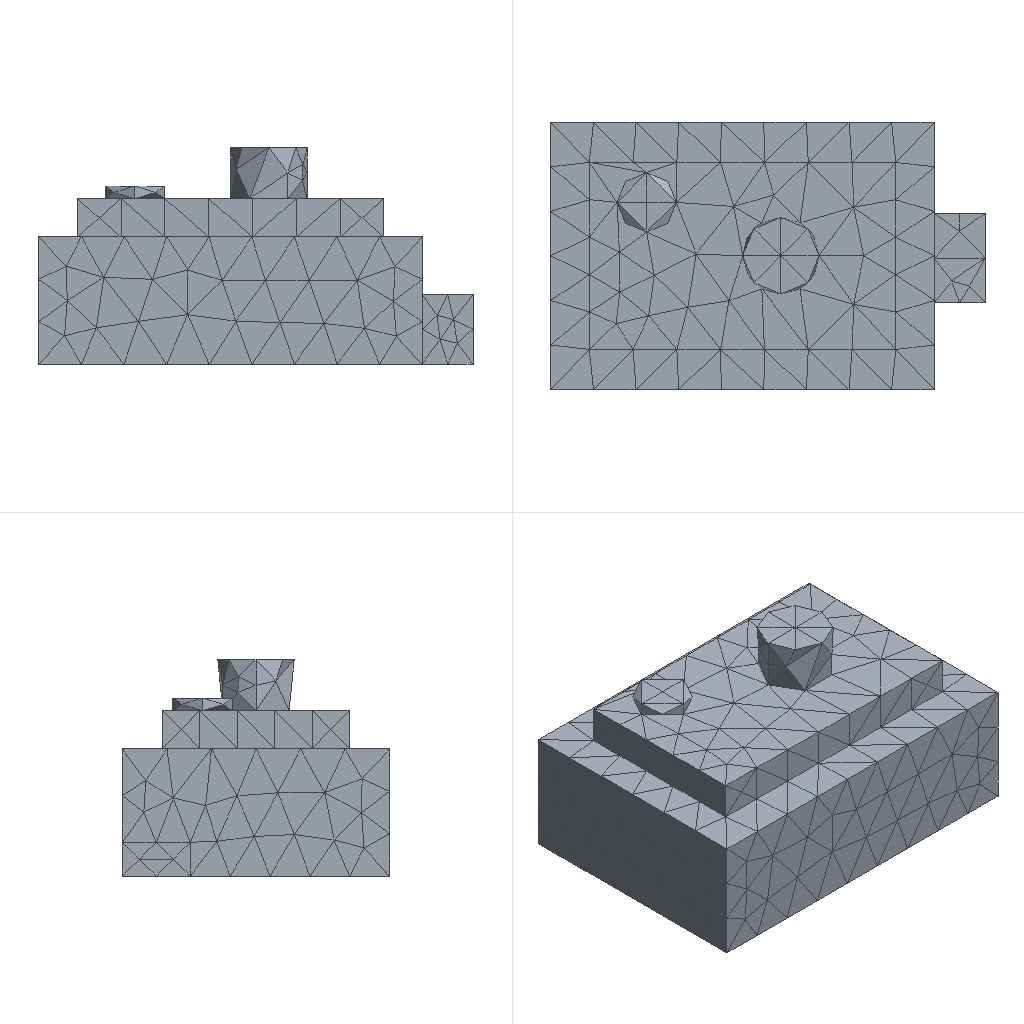Simulation study | ansys mapdl
Set-up summary:
category,name,step,type,value,unit,region
solver,ansys_mapdl
units,mm-N-s-tonne (MPa),,inferred,E=210000 density=
analysis,model,,static
mesh,nodes,,,3135
mesh,elements,,,1804
element_type,SOLID187,,,1804
material,mat 1,,E,210000
material,mat 1,,nu,0.3
load,,model,body load temp,,,all
load,,model,force,"1000 [dir=(0, 0, -1) n=135]",,node list
bc,,model,fixed,"[dofs=UX,UY,UZ n=3556]",,node list
Ansys APDL input file, long lists of numbers shortened:
/COM,ANSYS RELEASE 2026 R1           BUILD 26.1      UP20260202       09:09:04
/PREP7
/NOPR
/TITLE,2
ANTYPE, 0
*IF,_CDRDOFF,EQ,1,THEN     !if solid model was read in
_CDRDOFF=             !reset flag, numoffs already performed
*ELSE              !offset database for the following FE model
NUMOFF,NODE,     3135
NUMOFF,ELEM,     1804
NUMOFF,MAT ,        1
NUMOFF,TYPE,        1
*ENDIF
*SET,_RETURN ,  0.
*SET,_STATUS ,  0.
*SET,_UIQR   ,  135.
*SET,__FLOATPARAMETER__,  3135.
DOF,DELETE
ETBLOCK,        1,        1
(2i9,19a9)
        1      187        0        0        0        0        0        0        0        0        0        0        0        0        0        0        0        0        0        0        0
       -1
NBLOCK,6,SOLID,      3135,      3135
(3i9,6e21.13e3)
        1        0        0-2.9175000000000E+001 3.1500000000000E+001 8.0000000000000E+000
! (3134 more lines like these left out)
N,UNBL,LOC,       -1,
EBLOCK,19,SOLID,      1804,      1804
(19i10)
         1         1         1         1         0         0         0         0        10         0         1      1371      1372      1373      1374      1522      1523      1524      1525
! (3607 more lines like these left out)
        -1
MPTEMP,UNBL, 1, 1,  0.    ,
MPDATA,UNBL, 1,EX  ,       1, 1,  210000.000    ,
MPTEMP,UNBL, 1, 1,  0.    ,
MPDATA,UNBL, 1,NUXY,       1, 1, 0.3    ,
MPTEMP,UNBL, 1, 1,  0.    ,
MPDATA,UNBL, 1,PRXY,       1, 1, 0.3    ,
EXTOPT,ATTR,      0,      0,      0
EXTOPT,ESIZE,  0,  0.
EXTOPT,ACLEAR,      0
TREF,  0.
IRLF,  0
BFUNIF,TEMP,_TINY
ACEL,  0.    ,  0.    ,  0.
OMEGA,  0.    ,  0.    ,  0.
DOMEGA,  0.    ,  0.    ,  0.
CGLOC,  0.    ,  0.    ,  0.
CGOMEGA,  0.    ,  0.    ,  0.
DCGOMG,  0.    ,  0.    ,  0.
KUSE,     0
TIME,  0.
ALPHAD,  0.
BETAD,  0.
DMPRAT,  0.
DMPSTR,  0.
CRPLIM, 0.1    ,   0
CRPLIM,  0.    ,   1
NCNV,     0, 1.000000000E+12,     0,  0.    ,  0.
NEQIT,     0
ERESX,DEFA
DBLOCK,      3556
(i9,a6,2(pg16.9))
        1  UX    0.00000000      0.00000000
! (3555 more lines like these left out)
       -1
FBLOCK,       135
(i9,a6,2(pg16.9))
      650  FZ   -7.40740741      0.00000000
! (134 more lines like these left out)
       -1
/GO
FINISH
Results summary:
result,analysis_type_db,,,static,unstated
result,n_sets,,,1,unstated
result,load_steps[0].set,load_step=1,,1,unstated
result,load_steps[0].substep,load_step=1,,1,unstated
result,load_steps[0].time,load_step=1,,1,unstated
result,load_steps[0].freq,load_step=1,,1,unstated
result,load_steps[0].max_usum,load_step=1,,0.0003467,unstated
result,load_steps[0].max_seqv,load_step=1,,5.145,unstated
result,load_steps[0].reaction_sum.FX,load_step=1,,2.20099e-11,unstated
result,load_steps[0].reaction_sum.FY,load_step=1,,1.05391e-11,unstated
result,load_steps[0].reaction_sum.FZ,load_step=1,,1000,unstated
result,load_steps[0].reaction_sum.MX,load_step=1,,0,unstated
result,load_steps[0].reaction_sum.MY,load_step=1,,0,unstated
result,load_steps[0].reaction_sum.MZ,load_step=1,,0,unstated
result,convergence,,,results present for all listed sets,unstated